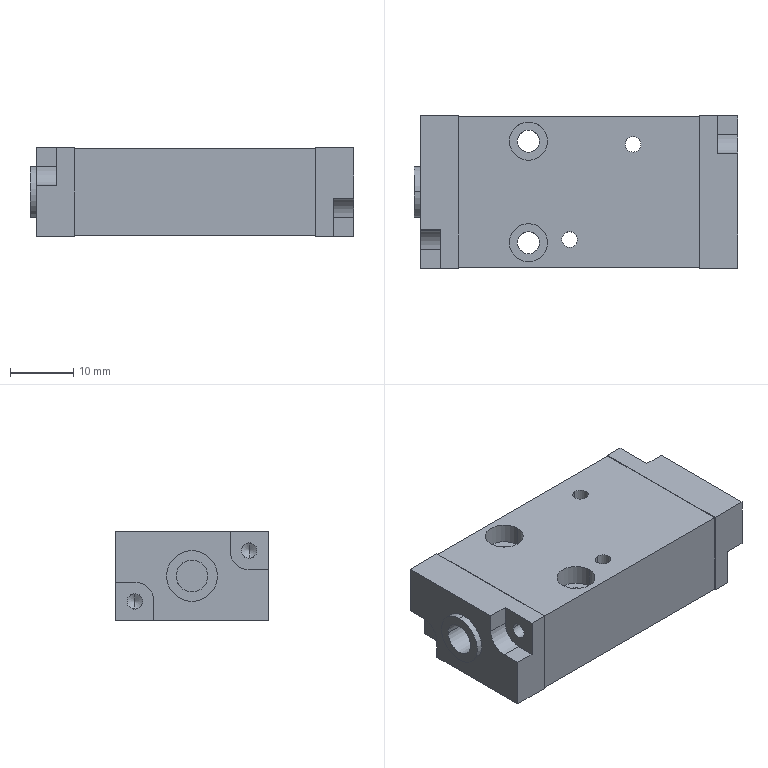Part | SolidWorks | features BaseBody 1 | 1 solid | 82 faces | box 51 x 24 x 14 mm | volume 14438 mm3 | cylinder 36 | plane 35 | cone 11 | commonest cylinder face diameters 2.459 x12 6 x12 3.5 x4 4.134 x4 5 x2 8 x2